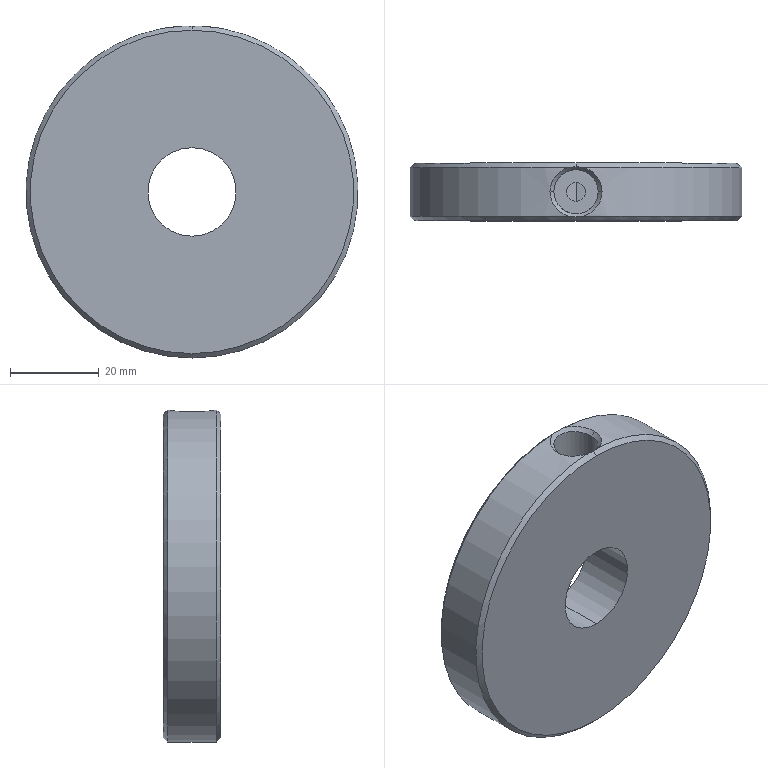Part | STEP file | QA-FC15 | 1 solid | 17 faces | box 75 x 13 x 74.963 mm | volume 51433 mm3 | cylinder 8 | cone 4 | plane 3 | spline 2 | commonest cylinder face diameters 4.2 x2 10 x2 20 x2 75 x2